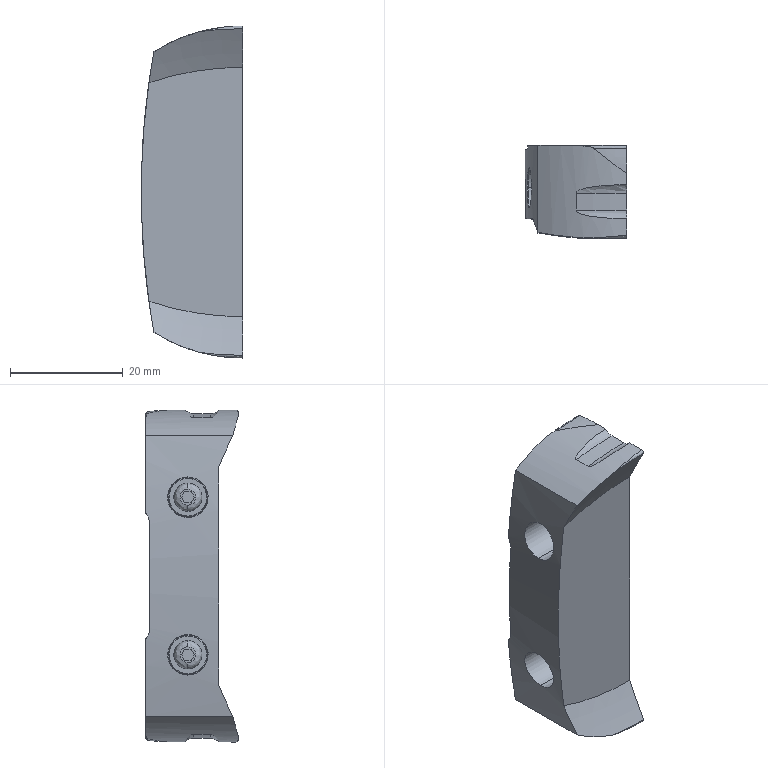Part | STEP file | _Gummipuffer-SBG - PAS42 B | 1 solid | 67 faces | box 18 x 16.46 x 59 mm | volume 11573 mm3 | plane 25 | spline 21 | cylinder 17 | torus 4 | commonest cylinder face diameters 5 x4 6.9 x4 7.2 x4 59 x2 116.6 x2 278 x1